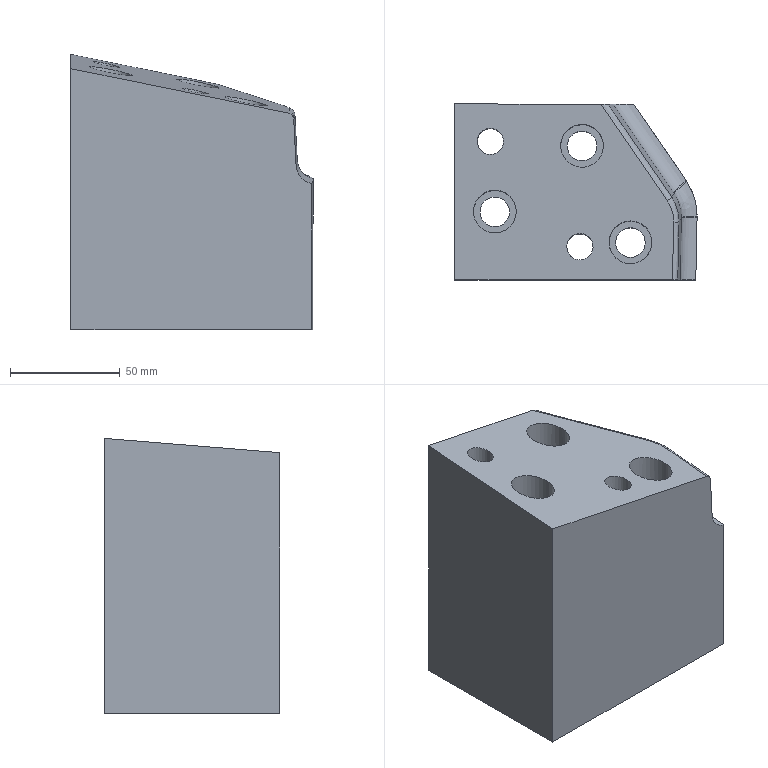Part | NX | features solid 2 | 1 solid | 30 faces | box 110.365 x 80 x 125.43 mm | volume 775159 mm3 | plane 11 | cylinder 11 | spline 8 | commonest cylinder face diameters 13.5 x3 19.5 x3 12 x2 18 x2 40 x1
STEP:
#1=CARTESIAN_POINT('',(-814.169,12.523,30.916));
#2=VERTEX_POINT('',#1);
#3=CARTESIAN_POINT('',(-838.426,48.,38.757));
#4=VERTEX_POINT('',#3);
#5=CARTESIAN_POINT('',(-814.169,12.523,30.916));
#6=CARTESIAN_POINT('',(-815.097,14.059,31.231));
#7=CARTESIAN_POINT('',(-817.162,16.985,31.89));
#8=CARTESIAN_POINT('',(-821.235,22.877,33.202));
#9=CARTESIAN_POINT('',(-826.296,30.263,34.836));
#10=CARTESIAN_POINT('',(-832.36,39.132,36.797));
#11=CARTESIAN_POINT('',(-836.404,45.044,38.104));
#12=CARTESIAN_POINT('',(-838.426,48.,38.757));
#13=B_SPLINE_CURVE_WITH_KNOTS('',3,(#5,#6,#7,#8,#9,#10,#11,#12),.UNSPECIFIED.,.F.,.F.,(4,1,1,1,1,4),(0.0458,0.05136,0.05692,0.06804,0.07916,0.09027),.UNSPECIFIED.);
#14=EDGE_CURVE('',#2,#4,#13,.T.);
#15=ORIENTED_EDGE('',*,*,#14,.T.);
#16=CARTESIAN_POINT('',(-814.56,13.109,31.044));
#17=VERTEX_POINT('',#16);
#18=CARTESIAN_POINT('',(-706.223,-145.27,-3.971));
#19=DIRECTION('',(0.5554,-0.812,-0.1795));
#20=VECTOR('',#19,1000.);
#21=LINE('',#18,#20);
#22=EDGE_CURVE('',#4,#17,#21,.T.);
#23=ORIENTED_EDGE('',*,*,#22,.T.);
#24=CARTESIAN_POINT('',(-838.989,-3.323,34.701));
#25=DIRECTION('',(-0.1996,0.07937,-0.9767));
#26=DIRECTION('',(0.9799,0.02089,-0.1986));
#27=AXIS2_PLACEMENT_3D('',#24,#25,#26);
#28=ELLIPSE('',#27,29.954,29.);
#29=EDGE_CURVE('',#17,#2,#28,.T.);
#30=ORIENTED_EDGE('',*,*,#29,.T.);
#31=EDGE_LOOP('',(#15,#23,#30));
#32=FACE_BOUND('',#31,.T.);
#33=CARTESIAN_POINT('',(-543.724,-28.864,-27.724));
#34=DIRECTION('',(-0.1996,0.07937,-0.9767));
#35=DIRECTION('',(0.9799,0.02089,-0.1986));
#36=AXIS2_PLACEMENT_3D('',#33,#34,#35);
#37=PLANE('',#36);
#38=ADVANCED_FACE('',(#32),#37,.F.);
#39=CARTESIAN_POINT('',(-857.279,-18.669,67.193));
#40=VERTEX_POINT('',#39);
#41=CARTESIAN_POINT('',(-859.902,-22.86,67.388));
#42=CARTESIAN_POINT('',(-856.633,-18.852,67.046));
#43=CARTESIAN_POINT('',(-857.243,-13.746,67.585));
#44=CARTESIAN_POINT('',(-861.169,-10.636,68.641));
#45=CARTESIAN_POINT('',(-866.18,-11.127,69.625));
#46=CARTESIAN_POINT('',(-869.446,-15.132,69.967));
#47=CARTESIAN_POINT('',(-868.843,-20.233,69.429));
#48=CARTESIAN_POINT('',(-864.913,-23.352,68.372));
#49=CARTESIAN_POINT('',(-859.902,-22.86,67.388));
#50=CARTESIAN_POINT('',(-856.633,-18.852,67.046));
#51=CARTESIAN_POINT('',(-857.243,-13.746,67.585));
#52=B_SPLINE_CURVE_WITH_KNOTS('',3,(#41,#42,#43,#44,#45,#46,#47,#48,#49,#50,#51),.UNSPECIFIED.,.T.,.F.,(1,1,1,1,1,1,1,1,1,1,1,1,1,1,1),(-0.01424,-0.009492,-0.004746,0.,0.004746,0.009492,0.01424,0.01898,0.02373,0.02848,0.03322,0.03797,0.04271,0.04746,0.05221),.UNSPECIFIED.);
#53=EDGE_CURVE('',#40,#40,#52,.T.);
#54=ORIENTED_EDGE('',*,*,#53,.F.);
#55=EDGE_LOOP('',(#54));
#56=FACE_BOUND('',#55,.T.);
#57=CARTESIAN_POINT('',(-909.709,-6.673,78.884));
#58=VERTEX_POINT('',#57);
#59=CARTESIAN_POINT('',(-903.612,-11.594,77.238));
#60=CARTESIAN_POINT('',(-910.538,-7.306,79.002));
#61=CARTESIAN_POINT('',(-912.489,0.7824,80.058));
#62=CARTESIAN_POINT('',(-908.008,7.886,79.719));
#63=CARTESIAN_POINT('',(-899.97,9.645,78.219));
#64=CARTESIAN_POINT('',(-893.065,5.359,76.46));
#65=CARTESIAN_POINT('',(-891.101,-2.711,75.402));
#66=CARTESIAN_POINT('',(-895.587,-9.835,75.74));
#67=CARTESIAN_POINT('',(-903.612,-11.594,77.238));
#68=CARTESIAN_POINT('',(-910.538,-7.306,79.002));
#69=CARTESIAN_POINT('',(-912.489,0.7824,80.058));
#70=B_SPLINE_CURVE_WITH_KNOTS('',3,(#59,#60,#61,#62,#63,#64,#65,#66,#67,#68,#69),.UNSPECIFIED.,.T.,.F.,(1,1,1,1,1,1,1,1,1,1,1,1,1,1,1),(-0.02314,-0.01542,-0.007712,0.,0.007712,0.01542,0.02314,0.03085,0.03856,0.04627,0.05398,0.06169,0.06941,0.07712,0.08483),.UNSPECIFIED.);
#71=EDGE_CURVE('',#58,#58,#70,.T.);
#72=ORIENTED_EDGE('',*,*,#71,.T.);
#73=EDGE_LOOP('',(#72));
#74=FACE_BOUND('',#73,.T.);
#75=CARTESIAN_POINT('',(-849.687,-16.103,65.849));
#76=VERTEX_POINT('',#75);
#77=CARTESIAN_POINT('',(-846.7,-23.44,64.643));
#78=CARTESIAN_POINT('',(-850.754,-16.253,66.055));
#79=CARTESIAN_POINT('',(-848.406,-8.168,66.232));
#80=CARTESIAN_POINT('',(-841.091,-4.27,65.054));
#81=CARTESIAN_POINT('',(-833.29,-6.567,63.273));
#82=CARTESIAN_POINT('',(-829.252,-13.743,61.864));
#83=CARTESIAN_POINT('',(-831.581,-21.819,61.684));
#84=CARTESIAN_POINT('',(-838.912,-25.731,62.864));
#85=CARTESIAN_POINT('',(-846.7,-23.44,64.643));
#86=CARTESIAN_POINT('',(-850.754,-16.253,66.055));
#87=CARTESIAN_POINT('',(-848.406,-8.168,66.232));
#88=B_SPLINE_CURVE_WITH_KNOTS('',3,(#77,#78,#79,#80,#81,#82,#83,#84,#85,#86,#87),.UNSPECIFIED.,.T.,.F.,(1,1,1,1,1,1,1,1,1,1,1,1,1,1,1),(-0.02314,-0.01543,-0.007713,0.,0.007713,0.01543,0.02314,0.03085,0.03857,0.04628,0.05399,0.06171,0.06942,0.07713,0.08485),.UNSPECIFIED.);
#89=EDGE_CURVE('',#76,#76,#88,.T.);
#90=ORIENTED_EDGE('',*,*,#89,.T.);
#91=EDGE_LOOP('',(#90));
#92=FACE_BOUND('',#91,.T.);
#93=CARTESIAN_POINT('',(-871.247,25.732,73.656));
#94=VERTEX_POINT('',#93);
#95=CARTESIAN_POINT('',(-866.719,19.289,72.207));
#96=CARTESIAN_POINT('',(-872.237,25.345,73.827));
#97=CARTESIAN_POINT('',(-871.815,33.724,74.421));
#98=CARTESIAN_POINT('',(-865.534,39.227,73.585));
#99=CARTESIAN_POINT('',(-857.389,38.706,71.878));
#100=CARTESIAN_POINT('',(-851.893,32.658,70.263));
#101=CARTESIAN_POINT('',(-852.296,24.292,69.666));
#102=CARTESIAN_POINT('',(-858.589,18.772,70.503));
#103=CARTESIAN_POINT('',(-866.719,19.289,72.207));
#104=CARTESIAN_POINT('',(-872.237,25.345,73.827));
#105=CARTESIAN_POINT('',(-871.815,33.724,74.421));
#106=B_SPLINE_CURVE_WITH_KNOTS('',3,(#95,#96,#97,#98,#99,#100,#101,#102,#103,#104,#105),.UNSPECIFIED.,.T.,.F.,(1,1,1,1,1,1,1,1,1,1,1,1,1,1,1),(-0.02314,-0.01543,-0.007713,0.,0.007713,0.01543,0.02314,0.03085,0.03856,0.04628,0.05399,0.0617,0.06942,0.07713,0.08484),.UNSPECIFIED.);
#107=EDGE_CURVE('',#94,#94,#106,.T.);
#108=ORIENTED_EDGE('',*,*,#107,.T.);
#109=EDGE_LOOP('',(#108));
#110=FACE_BOUND('',#109,.T.);
#111=CARTESIAN_POINT('',(-908.757,34.366,82.024));
#112=VERTEX_POINT('',#111);
#113=CARTESIAN_POINT('',(-904.976,37.499,81.506));
#114=CARTESIAN_POINT('',(-909.304,34.754,82.168));
#115=CARTESIAN_POINT('',(-910.352,29.683,81.97));
#116=CARTESIAN_POINT('',(-907.547,25.48,81.055));
#117=CARTESIAN_POINT('',(-902.655,24.423,79.969));
#118=CARTESIAN_POINT('',(-898.335,27.166,79.309));
#119=CARTESIAN_POINT('',(-897.28,32.228,79.505));
#120=CARTESIAN_POINT('',(-900.089,36.443,80.421));
#121=CARTESIAN_POINT('',(-904.976,37.499,81.506));
#122=CARTESIAN_POINT('',(-909.304,34.754,82.168));
#123=CARTESIAN_POINT('',(-910.352,29.683,81.97));
#124=B_SPLINE_CURVE_WITH_KNOTS('',3,(#113,#114,#115,#116,#117,#118,#119,#120,#121,#122,#123),.UNSPECIFIED.,.T.,.F.,(1,1,1,1,1,1,1,1,1,1,1,1,1,1,1),(-0.01424,-0.009493,-0.004747,0.,0.004747,0.009493,0.01424,0.01899,0.02373,0.02848,0.03323,0.03797,0.04272,0.04747,0.05221),.UNSPECIFIED.);
#125=EDGE_CURVE('',#112,#112,#124,.T.);
#126=ORIENTED_EDGE('',*,*,#125,.F.);
#127=EDGE_LOOP('',(#126));
#128=FACE_BOUND('',#127,.T.);
#129=CARTESIAN_POINT('',(-820.85,-32.,58.663));
#130=VERTEX_POINT('',#129);
#131=CARTESIAN_POINT('',(-920.,-32.,78.929));
#132=VERTEX_POINT('',#131);
#133=CARTESIAN_POINT('',(-820.85,-32.,58.663));
#134=CARTESIAN_POINT('',(-853.9,-32.,65.419));
#135=CARTESIAN_POINT('',(-886.95,-32.,72.174));
#136=CARTESIAN_POINT('',(-920.,-32.,78.929));
#137=B_SPLINE_CURVE_WITH_KNOTS('',3,(#133,#134,#135,#136),.UNSPECIFIED.,.F.,.F.,(4,4),(0.,0.1012),.UNSPECIFIED.);
#138=EDGE_CURVE('',#130,#132,#137,.T.);
#139=ORIENTED_EDGE('',*,*,#138,.F.);
#140=CARTESIAN_POINT('',(-820.322,-5.789,60.686));
#141=VERTEX_POINT('',#140);
#142=CARTESIAN_POINT('',(-820.85,-32.,58.663));
#143=CARTESIAN_POINT('',(-820.674,-23.263,59.337));
#144=CARTESIAN_POINT('',(-820.498,-14.526,60.011));
#145=CARTESIAN_POINT('',(-820.322,-5.789,60.686));
#146=B_SPLINE_CURVE_WITH_KNOTS('',3,(#142,#143,#144,#145),.UNSPECIFIED.,.F.,.F.,(4,4),(0.,0.02629),.UNSPECIFIED.);
#147=EDGE_CURVE('',#130,#141,#146,.T.);
#148=ORIENTED_EDGE('',*,*,#147,.T.);
#149=CARTESIAN_POINT('',(-823.204,3.891,62.061));
#150=VERTEX_POINT('',#149);
#151=CARTESIAN_POINT('',(-820.322,-5.789,60.686));
#152=CARTESIAN_POINT('',(-820.252,-2.318,60.953));
#153=CARTESIAN_POINT('',(-821.27,1.064,61.436));
#154=CARTESIAN_POINT('',(-823.204,3.891,62.061));
#155=B_SPLINE_CURVE_WITH_KNOTS('',3,(#151,#152,#153,#154),.UNSPECIFIED.,.F.,.F.,(4,4),(0.,0.01034),.UNSPECIFIED.);
#156=EDGE_CURVE('',#141,#150,#155,.T.);
#157=ORIENTED_EDGE('',*,*,#156,.T.);
#158=CARTESIAN_POINT('',(-853.376,48.,71.813));
#159=VERTEX_POINT('',#158);
#160=CARTESIAN_POINT('',(-823.204,3.891,62.061));
#161=CARTESIAN_POINT('',(-833.261,18.594,65.312));
#162=CARTESIAN_POINT('',(-843.319,33.297,68.562));
#163=CARTESIAN_POINT('',(-853.376,48.,71.813));
#164=B_SPLINE_CURVE_WITH_KNOTS('',3,(#160,#161,#162,#163),.UNSPECIFIED.,.F.,.F.,(4,4),(0.,0.05432),.UNSPECIFIED.);
#165=EDGE_CURVE('',#150,#159,#164,.T.);
#166=ORIENTED_EDGE('',*,*,#165,.T.);
#167=CARTESIAN_POINT('',(-920.,48.,85.43));
#168=VERTEX_POINT('',#167);
#169=CARTESIAN_POINT('',(-853.376,48.,71.813));
#170=CARTESIAN_POINT('',(-875.584,48.,76.352));
#171=CARTESIAN_POINT('',(-897.792,48.,80.891));
#172=CARTESIAN_POINT('',(-920.,48.,85.43));
#173=B_SPLINE_CURVE_WITH_KNOTS('',3,(#169,#170,#171,#172),.UNSPECIFIED.,.F.,.F.,(4,4),(0.1961,0.2641),.UNSPECIFIED.);
#174=EDGE_CURVE('',#159,#168,#173,.T.);
#175=ORIENTED_EDGE('',*,*,#174,.T.);
#176=CARTESIAN_POINT('',(-920.,-32.,78.929));
#177=CARTESIAN_POINT('',(-920.,-5.333,81.096));
#178=CARTESIAN_POINT('',(-920.,21.333,83.263));
#179=CARTESIAN_POINT('',(-920.,48.,85.43));
#180=B_SPLINE_CURVE_WITH_KNOTS('',3,(#176,#177,#178,#179),.UNSPECIFIED.,.F.,.F.,(4,4),(0.,0.08026),.UNSPECIFIED.);
#181=EDGE_CURVE('',#132,#168,#180,.T.);
#182=ORIENTED_EDGE('',*,*,#181,.F.);
#183=EDGE_LOOP('',(#139,#148,#157,#166,#175,#182));
#184=FACE_BOUND('',#183,.T.);
#185=CARTESIAN_POINT('',(-920.974,48.472,85.668));
#186=CARTESIAN_POINT('',(-920.587,-34.619,78.836));
#187=CARTESIAN_POINT('',(-919.909,48.495,85.452));
#188=CARTESIAN_POINT('',(-919.523,-34.596,78.62));
#189=CARTESIAN_POINT('',(-900.858,48.901,81.591));
#190=CARTESIAN_POINT('',(-900.471,-34.19,74.759));
#191=CARTESIAN_POINT('',(-869.11,49.577,75.157));
#192=CARTESIAN_POINT('',(-868.723,-33.513,68.325));
#193=CARTESIAN_POINT('',(-819.947,50.626,65.194));
#194=CARTESIAN_POINT('',(-819.56,-32.465,58.362));
#195=B_SPLINE_SURFACE_WITH_KNOTS('',1,1,((#185,#186),(#187,#188),(#189,#190),(#191,#192),(#193,#194)),.PLANE_SURF.,.F.,.F.,.F.,(2,1,1,1,2),(2,2),(-0.2849,-0.2791,-0.1744,0.,0.2701),(0.3913,0.7679),.PIECEWISE_BEZIER_KNOTS.);
#196=ADVANCED_FACE('',(#56,#74,#92,#110,#128,#184),#195,.F.);
#197=CARTESIAN_POINT('',(-838.426,48.,-40.));
#198=VERTEX_POINT('',#197);
#199=CARTESIAN_POINT('',(-838.426,48.,-20.));
#200=DIRECTION('',(0.,0.,1.));
#201=VECTOR('',#200,1000.);
#202=LINE('',#199,#201);
#203=EDGE_CURVE('',#4,#198,#202,.F.);
#204=ORIENTED_EDGE('',*,*,#203,.F.);
#205=ORIENTED_EDGE('',*,*,#14,.F.);
#206=CARTESIAN_POINT('',(-809.639,-2.963,28.732));
#207=VERTEX_POINT('',#206);
#208=CARTESIAN_POINT('',(-809.639,-2.963,28.732));
#209=CARTESIAN_POINT('',(-809.665,-0.1967,28.962));
#210=CARTESIAN_POINT('',(-810.39,5.202,29.549));
#211=CARTESIAN_POINT('',(-812.779,10.219,30.445));
#212=CARTESIAN_POINT('',(-814.169,12.523,30.916));
#213=B_SPLINE_CURVE_WITH_KNOTS('',3,(#208,#209,#210,#211,#212),.UNSPECIFIED.,.F.,.F.,(4,1,4),(0.02913,0.03746,0.0458),.UNSPECIFIED.);
#214=EDGE_CURVE('',#207,#2,#213,.T.);
#215=ORIENTED_EDGE('',*,*,#214,.F.);
#216=CARTESIAN_POINT('',(-810.22,-32.,26.491));
#217=VERTEX_POINT('',#216);
#218=CARTESIAN_POINT('',(-810.22,-32.,26.491));
#219=CARTESIAN_POINT('',(-810.123,-27.16,26.864));
#220=CARTESIAN_POINT('',(-809.961,-19.9,27.421));
#221=CARTESIAN_POINT('',(-809.807,-10.223,28.176));
#222=CARTESIAN_POINT('',(-809.615,-5.38,28.53));
#223=CARTESIAN_POINT('',(-809.639,-2.963,28.732));
#224=B_SPLINE_CURVE_WITH_KNOTS('',3,(#218,#219,#220,#221,#222,#223),.UNSPECIFIED.,.F.,.F.,(4,1,1,4),(0.,0.01456,0.02185,0.02913),.UNSPECIFIED.);
#225=EDGE_CURVE('',#217,#207,#224,.T.);
#226=ORIENTED_EDGE('',*,*,#225,.F.);
#227=CARTESIAN_POINT('',(-810.22,-32.,-40.));
#228=VERTEX_POINT('',#227);
#229=CARTESIAN_POINT('',(-810.22,-32.,-20.));
#230=DIRECTION('',(0.,0.,1.));
#231=VECTOR('',#230,1000.);
#232=LINE('',#229,#231);
#233=EDGE_CURVE('',#217,#228,#232,.F.);
#234=ORIENTED_EDGE('',*,*,#233,.T.);
#235=CARTESIAN_POINT('',(-810.22,-32.,-40.));
#236=CARTESIAN_POINT('',(-810.146,-28.288,-40.));
#237=CARTESIAN_POINT('',(-810.036,-22.72,-40.));
#238=CARTESIAN_POINT('',(-809.879,-15.297,-40.));
#239=CARTESIAN_POINT('',(-809.787,-9.727,-40.));
#240=CARTESIAN_POINT('',(-809.579,-4.166,-40.));
#241=CARTESIAN_POINT('',(-809.762,1.427,-40.));
#242=CARTESIAN_POINT('',(-811.176,6.752,-40.));
#243=CARTESIAN_POINT('',(-813.579,11.806,-40.));
#244=CARTESIAN_POINT('',(-816.679,16.319,-40.));
#245=CARTESIAN_POINT('',(-819.822,20.825,-40.));
#246=CARTESIAN_POINT('',(-822.929,25.349,-40.));
#247=CARTESIAN_POINT('',(-827.065,31.388,-40.));
#248=CARTESIAN_POINT('',(-832.228,38.939,-40.));
#249=CARTESIAN_POINT('',(-836.36,44.98,-40.));
#250=CARTESIAN_POINT('',(-838.426,48.,-40.));
#251=B_SPLINE_CURVE_WITH_KNOTS('',3,(#235,#236,#237,#238,#239,#240,#241,#242,#243,#244,#245,#246,#247,#248,#249,#250),.UNSPECIFIED.,.F.,.F.,(4,1,1,1,1,1,1,1,1,1,1,1,1,4),(0.,0.01114,0.01671,0.02228,0.02784,0.03341,0.03898,0.04455,0.05012,0.05569,0.06126,0.06683,0.07797,0.0891),.UNSPECIFIED.);
#252=EDGE_CURVE('',#228,#198,#251,.T.);
#253=ORIENTED_EDGE('',*,*,#252,.T.);
#254=EDGE_LOOP('',(#204,#205,#215,#226,#234,#253));
#255=FACE_BOUND('',#254,.T.);
#256=CARTESIAN_POINT('',(-838.426,48.,-40.));
#257=CARTESIAN_POINT('',(-838.426,48.,39.23));
#258=CARTESIAN_POINT('',(-834.685,42.53,-40.));
#259=CARTESIAN_POINT('',(-834.685,42.53,39.23));
#260=CARTESIAN_POINT('',(-827.52,32.055,-40.));
#261=CARTESIAN_POINT('',(-827.52,32.055,39.23));
#262=CARTESIAN_POINT('',(-819.564,20.425,-40.));
#263=CARTESIAN_POINT('',(-819.564,20.425,39.23));
#264=CARTESIAN_POINT('',(-813.609,11.918,-40.));
#265=CARTESIAN_POINT('',(-813.609,11.918,39.23));
#266=CARTESIAN_POINT('',(-811.044,6.684,-40.));
#267=CARTESIAN_POINT('',(-811.044,6.684,39.23));
#268=CARTESIAN_POINT('',(-809.788,0.9757,-40.));
#269=CARTESIAN_POINT('',(-809.788,0.9757,39.23));
#270=CARTESIAN_POINT('',(-809.603,-2.547,-40.));
#271=CARTESIAN_POINT('',(-809.603,-2.547,39.23));
#272=CARTESIAN_POINT('',(-809.753,-8.818,-40.));
#273=CARTESIAN_POINT('',(-809.753,-8.818,39.23));
#274=CARTESIAN_POINT('',(-809.945,-18.35,-40.));
#275=CARTESIAN_POINT('',(-809.945,-18.35,39.23));
#276=CARTESIAN_POINT('',(-810.125,-27.28,-40.));
#277=CARTESIAN_POINT('',(-810.125,-27.28,39.23));
#278=CARTESIAN_POINT('',(-810.22,-32.,-40.));
#279=CARTESIAN_POINT('',(-810.22,-32.,39.23));
#280=B_SPLINE_SURFACE_WITH_KNOTS('',3,1,((#256,#257),(#258,#259),(#260,#261),(#262,#263),(#264,#265),(#266,#267),(#268,#269),(#270,#271),(#272,#273),(#274,#275),(#276,#277),(#278,#279)),.SURF_OF_LINEAR_EXTRUSION.,.F.,.F.,.F.,(4,1,1,1,1,1,1,1,1,4),(2,2),(0.4314,0.463,0.492,0.4987,0.5127,0.5196,0.5266,0.5295,0.5496,0.5722),(0.4274,0.7151),.UNSPECIFIED.);
#281=ADVANCED_FACE('',(#255),#280,.F.);
#282=ORIENTED_EDGE('',*,*,#174,.F.);
#283=CARTESIAN_POINT('',(-850.192,48.,68.733));
#284=VERTEX_POINT('',#283);
#285=CARTESIAN_POINT('',(-853.376,48.,71.813));
#286=CARTESIAN_POINT('',(-852.599,48.,71.654));
#287=CARTESIAN_POINT('',(-851.15,48.,70.951));
#288=CARTESIAN_POINT('',(-850.277,48.,69.525));
#289=CARTESIAN_POINT('',(-850.192,48.,68.733));
#290=B_SPLINE_CURVE_WITH_KNOTS('',3,(#285,#286,#287,#288,#289),.UNSPECIFIED.,.F.,.F.,(4,1,4),(0.,0.002346,0.004693),.UNSPECIFIED.);
#291=EDGE_CURVE('',#159,#284,#290,.T.);
#292=ORIENTED_EDGE('',*,*,#291,.T.);
#293=CARTESIAN_POINT('',(-847.978,48.,47.999));
#294=VERTEX_POINT('',#293);
#295=CARTESIAN_POINT('',(-838.657,48.,-39.294));
#296=DIRECTION('',(-0.1062,0.,0.9943));
#297=VECTOR('',#296,1000.);
#298=LINE('',#295,#297);
#299=EDGE_CURVE('',#284,#294,#298,.F.);
#300=ORIENTED_EDGE('',*,*,#299,.T.);
#301=CARTESIAN_POINT('',(-837.118,48.,47.705));
#302=DIRECTION('',(0.,1.,0.));
#303=DIRECTION('',(-0.9515,0.,0.3075));
#304=AXIS2_PLACEMENT_3D('',#301,#302,#303);
#305=ELLIPSE('',#304,11.084,9.);
#306=EDGE_CURVE('',#294,#4,#305,.F.);
#307=ORIENTED_EDGE('',*,*,#306,.T.);
#308=ORIENTED_EDGE('',*,*,#203,.T.);
#309=CARTESIAN_POINT('',(-920.,48.,-40.));
#310=VERTEX_POINT('',#309);
#311=CARTESIAN_POINT('',(-813.69,48.,-40.));
#312=DIRECTION('',(1.,0.,0.));
#313=VECTOR('',#312,1000.);
#314=LINE('',#311,#313);
#315=EDGE_CURVE('',#198,#310,#314,.F.);
#316=ORIENTED_EDGE('',*,*,#315,.T.);
#317=CARTESIAN_POINT('',(-920.,48.,100.));
#318=DIRECTION('',(0.,0.,1.));
#319=VECTOR('',#318,1000.);
#320=LINE('',#317,#319);
#321=EDGE_CURVE('',#168,#310,#320,.F.);
#322=ORIENTED_EDGE('',*,*,#321,.F.);
#323=EDGE_LOOP('',(#282,#292,#300,#307,#308,#316,#322));
#324=FACE_BOUND('',#323,.T.);
#325=CARTESIAN_POINT('',(-915.5,48.,-47.5));
#326=DIRECTION('',(0.,1.,0.));
#327=DIRECTION('',(-1.,0.,0.));
#328=AXIS2_PLACEMENT_3D('',#325,#326,#327);
#329=PLANE('',#328);
#330=ADVANCED_FACE('',(#324),#329,.T.);
#331=CARTESIAN_POINT('',(-817.4,-32.,34.867));
#332=VERTEX_POINT('',#331);
#333=CARTESIAN_POINT('',(-818.457,-32.,55.871));
#334=VERTEX_POINT('',#333);
#335=CARTESIAN_POINT('',(-813.512,-32.,-42.366));
#336=DIRECTION('',(0.05028,0.,-0.9987));
#337=VECTOR('',#336,1000.);
#338=LINE('',#335,#337);
#339=EDGE_CURVE('',#332,#334,#338,.F.);
#340=ORIENTED_EDGE('',*,*,#339,.T.);
#341=CARTESIAN_POINT('',(-818.457,-32.,55.871));
#342=CARTESIAN_POINT('',(-818.524,-32.,57.201));
#343=CARTESIAN_POINT('',(-819.546,-32.,58.397));
#344=CARTESIAN_POINT('',(-820.85,-32.,58.663));
#345=B_SPLINE_CURVE_WITH_KNOTS('',3,(#341,#342,#343,#344),.UNSPECIFIED.,.F.,.F.,(4,4),(0.,0.003938),.UNSPECIFIED.);
#346=EDGE_CURVE('',#334,#130,#345,.T.);
#347=ORIENTED_EDGE('',*,*,#346,.T.);
#348=ORIENTED_EDGE('',*,*,#138,.T.);
#349=CARTESIAN_POINT('',(-920.,-32.,-40.));
#350=VERTEX_POINT('',#349);
#351=CARTESIAN_POINT('',(-920.,-32.,100.));
#352=DIRECTION('',(0.,0.,-1.));
#353=VECTOR('',#352,1000.);
#354=LINE('',#351,#353);
#355=EDGE_CURVE('',#132,#350,#354,.T.);
#356=ORIENTED_EDGE('',*,*,#355,.T.);
#357=CARTESIAN_POINT('',(-813.69,-32.,-40.));
#358=DIRECTION('',(-1.,0.,0.));
#359=VECTOR('',#358,1000.);
#360=LINE('',#357,#359);
#361=EDGE_CURVE('',#228,#350,#360,.T.);
#362=ORIENTED_EDGE('',*,*,#361,.F.);
#363=ORIENTED_EDGE('',*,*,#233,.F.);
#364=CARTESIAN_POINT('',(-808.409,-32.,35.336));
#365=DIRECTION('',(0.,-1.,0.));
#366=DIRECTION('',(0.2528,0.,0.9675));
#367=AXIS2_PLACEMENT_3D('',#364,#365,#366);
#368=ELLIPSE('',#367,9.029,9.);
#369=EDGE_CURVE('',#217,#332,#368,.F.);
#370=ORIENTED_EDGE('',*,*,#369,.T.);
#371=EDGE_LOOP('',(#340,#347,#348,#356,#362,#363,#370));
#372=FACE_BOUND('',#371,.T.);
#373=CARTESIAN_POINT('',(-915.5,-32.,-47.5));
#374=DIRECTION('',(0.,-1.,0.));
#375=DIRECTION('',(1.,0.,0.));
#376=AXIS2_PLACEMENT_3D('',#373,#374,#375);
#377=PLANE('',#376);
#378=ADVANCED_FACE('',(#372),#377,.T.);
#379=ORIENTED_EDGE('',*,*,#252,.F.);
#380=ORIENTED_EDGE('',*,*,#361,.T.);
#381=CARTESIAN_POINT('',(-920.,-31.695,-40.));
#382=DIRECTION('',(0.,1.,0.));
#383=VECTOR('',#382,1000.);
#384=LINE('',#381,#383);
#385=EDGE_CURVE('',#350,#310,#384,.T.);
#386=ORIENTED_EDGE('',*,*,#385,.T.);
#387=ORIENTED_EDGE('',*,*,#315,.F.);
#388=EDGE_LOOP('',(#379,#380,#386,#387));
#389=FACE_BOUND('',#388,.T.);
#390=CARTESIAN_POINT('',(-869.041,-16.993,-40.));
#391=VERTEX_POINT('',#390);
#392=CARTESIAN_POINT('',(-863.041,-16.993,-40.));
#393=DIRECTION('',(0.,0.,-1.));
#394=DIRECTION('',(-1.,0.,0.));
#395=AXIS2_PLACEMENT_3D('',#392,#393,#394);
#396=CIRCLE('',#395,6.);
#397=EDGE_CURVE('',#391,#391,#396,.F.);
#398=ORIENTED_EDGE('',*,*,#397,.T.);
#399=EDGE_LOOP('',(#398));
#400=FACE_BOUND('',#399,.T.);
#401=CARTESIAN_POINT('',(-908.547,-0.9737,-40.));
#402=VERTEX_POINT('',#401);
#403=CARTESIAN_POINT('',(-901.797,-0.9737,-40.));
#404=DIRECTION('',(0.,0.,-1.));
#405=DIRECTION('',(-1.,0.,0.));
#406=AXIS2_PLACEMENT_3D('',#403,#404,#405);
#407=CIRCLE('',#406,6.75);
#408=EDGE_CURVE('',#402,#402,#407,.T.);
#409=ORIENTED_EDGE('',*,*,#408,.F.);
#410=EDGE_LOOP('',(#409));
#411=FACE_BOUND('',#410,.T.);
#412=CARTESIAN_POINT('',(-846.75,-15.,-40.));
#413=VERTEX_POINT('',#412);
#414=CARTESIAN_POINT('',(-840.,-15.,-40.));
#415=DIRECTION('',(0.,0.,-1.));
#416=DIRECTION('',(-1.,0.,0.));
#417=AXIS2_PLACEMENT_3D('',#414,#415,#416);
#418=CIRCLE('',#417,6.75);
#419=EDGE_CURVE('',#413,#413,#418,.T.);
#420=ORIENTED_EDGE('',*,*,#419,.F.);
#421=EDGE_LOOP('',(#420));
#422=FACE_BOUND('',#421,.T.);
#423=CARTESIAN_POINT('',(-868.811,29.,-40.));
#424=VERTEX_POINT('',#423);
#425=CARTESIAN_POINT('',(-862.061,29.,-40.));
#426=DIRECTION('',(0.,0.,-1.));
#427=DIRECTION('',(-1.,0.,0.));
#428=AXIS2_PLACEMENT_3D('',#425,#426,#427);
#429=CIRCLE('',#428,6.75);
#430=EDGE_CURVE('',#424,#424,#429,.T.);
#431=ORIENTED_EDGE('',*,*,#430,.F.);
#432=EDGE_LOOP('',(#431));
#433=FACE_BOUND('',#432,.T.);
#434=CARTESIAN_POINT('',(-909.818,30.961,-40.));
#435=VERTEX_POINT('',#434);
#436=CARTESIAN_POINT('',(-903.818,30.961,-40.));
#437=DIRECTION('',(0.,0.,-1.));
#438=DIRECTION('',(-1.,0.,0.));
#439=AXIS2_PLACEMENT_3D('',#436,#437,#438);
#440=CIRCLE('',#439,6.);
#441=EDGE_CURVE('',#435,#435,#440,.F.);
#442=ORIENTED_EDGE('',*,*,#441,.T.);
#443=EDGE_LOOP('',(#442));
#444=FACE_BOUND('',#443,.T.);
#445=CARTESIAN_POINT('',(-813.69,4.103,-40.));
#446=DIRECTION('',(0.,0.,-1.));
#447=DIRECTION('',(-1.,0.,0.));
#448=AXIS2_PLACEMENT_3D('',#445,#446,#447);
#449=PLANE('',#448);
#450=ADVANCED_FACE('',(#389,#400,#411,#422,#433,#444),#449,.T.);
#451=ORIENTED_EDGE('',*,*,#385,.F.);
#452=ORIENTED_EDGE('',*,*,#355,.F.);
#453=ORIENTED_EDGE('',*,*,#181,.T.);
#454=ORIENTED_EDGE('',*,*,#321,.T.);
#455=EDGE_LOOP('',(#451,#452,#453,#454));
#456=FACE_BOUND('',#455,.T.);
#457=CARTESIAN_POINT('',(-920.,-31.695,100.));
#458=DIRECTION('',(1.,0.,0.));
#459=DIRECTION('',(0.,0.,1.));
#460=AXIS2_PLACEMENT_3D('',#457,#458,#459);
#461=PLANE('',#460);
#462=ADVANCED_FACE('',(#456),#461,.F.);
#463=CARTESIAN_POINT('',(-871.811,29.,-25.));
#464=VERTEX_POINT('',#463);
#465=CARTESIAN_POINT('',(-862.061,29.,-25.));
#466=DIRECTION('',(0.,0.,-1.));
#467=DIRECTION('',(-1.,0.,0.));
#468=AXIS2_PLACEMENT_3D('',#465,#466,#467);
#469=CIRCLE('',#468,9.75);
#470=EDGE_CURVE('',#464,#464,#469,.F.);
#471=ORIENTED_EDGE('',*,*,#470,.F.);
#472=EDGE_LOOP('',(#471));
#473=FACE_BOUND('',#472,.T.);
#474=ORIENTED_EDGE('',*,*,#107,.F.);
#475=EDGE_LOOP('',(#474));
#476=FACE_BOUND('',#475,.T.);
#477=CARTESIAN_POINT('',(-862.061,29.,-26.006));
#478=DIRECTION('',(0.,0.,1.));
#479=DIRECTION('',(1.,0.,0.));
#480=AXIS2_PLACEMENT_3D('',#477,#478,#479);
#481=CYLINDRICAL_SURFACE('',#480,9.75);
#482=ADVANCED_FACE('',(#473,#476),#481,.F.);
#483=ORIENTED_EDGE('',*,*,#430,.T.);
#484=EDGE_LOOP('',(#483));
#485=FACE_BOUND('',#484,.T.);
#486=CARTESIAN_POINT('',(-868.811,29.,-25.));
#487=VERTEX_POINT('',#486);
#488=CARTESIAN_POINT('',(-862.061,29.,-25.));
#489=DIRECTION('',(0.,0.,-1.));
#490=DIRECTION('',(-1.,0.,0.));
#491=AXIS2_PLACEMENT_3D('',#488,#489,#490);
#492=CIRCLE('',#491,6.75);
#493=EDGE_CURVE('',#487,#487,#492,.F.);
#494=ORIENTED_EDGE('',*,*,#493,.T.);
#495=EDGE_LOOP('',(#494));
#496=FACE_BOUND('',#495,.T.);
#497=CARTESIAN_POINT('',(-862.061,29.,-56.006));
#498=DIRECTION('',(0.,0.,1.));
#499=DIRECTION('',(1.,0.,0.));
#500=AXIS2_PLACEMENT_3D('',#497,#498,#499);
#501=CYLINDRICAL_SURFACE('',#500,6.75);
#502=ADVANCED_FACE('',(#485,#496),#501,.F.);
#503=ORIENTED_EDGE('',*,*,#493,.F.);
#504=EDGE_LOOP('',(#503));
#505=FACE_BOUND('',#504,.T.);
#506=ORIENTED_EDGE('',*,*,#470,.T.);
#507=EDGE_LOOP('',(#506));
#508=FACE_BOUND('',#507,.T.);
#509=CARTESIAN_POINT('',(-863.613,34.418,-25.));
#510=DIRECTION('',(0.,0.,-1.));
#511=DIRECTION('',(-1.,0.,0.));
#512=AXIS2_PLACEMENT_3D('',#509,#510,#511);
#513=PLANE('',#512);
#514=ADVANCED_FACE('',(#505,#508),#513,.F.);
#515=CARTESIAN_POINT('',(-830.25,-15.,-25.));
#516=VERTEX_POINT('',#515);
#517=CARTESIAN_POINT('',(-840.,-15.,-25.));
#518=DIRECTION('',(0.,0.,1.));
#519=DIRECTION('',(1.,0.,0.));
#520=AXIS2_PLACEMENT_3D('',#517,#518,#519);
#521=CIRCLE('',#520,9.75);
#522=EDGE_CURVE('',#516,#516,#521,.T.);
#523=ORIENTED_EDGE('',*,*,#522,.F.);
#524=EDGE_LOOP('',(#523));
#525=FACE_BOUND('',#524,.T.);
#526=ORIENTED_EDGE('',*,*,#89,.F.);
#527=EDGE_LOOP('',(#526));
#528=FACE_BOUND('',#527,.T.);
#529=CARTESIAN_POINT('',(-840.,-15.,-25.));
#530=DIRECTION('',(0.,0.,1.));
#531=DIRECTION('',(1.,0.,0.));
#532=AXIS2_PLACEMENT_3D('',#529,#530,#531);
#533=CYLINDRICAL_SURFACE('',#532,9.75);
#534=ADVANCED_FACE('',(#525,#528),#533,.F.);
#535=ORIENTED_EDGE('',*,*,#419,.T.);
#536=EDGE_LOOP('',(#535));
#537=FACE_BOUND('',#536,.T.);
#538=CARTESIAN_POINT('',(-846.75,-15.,-25.));
#539=VERTEX_POINT('',#538);
#540=CARTESIAN_POINT('',(-840.,-15.,-25.));
#541=DIRECTION('',(0.,0.,-1.));
#542=DIRECTION('',(-1.,0.,0.));
#543=AXIS2_PLACEMENT_3D('',#540,#541,#542);
#544=CIRCLE('',#543,6.75);
#545=EDGE_CURVE('',#539,#539,#544,.F.);
#546=ORIENTED_EDGE('',*,*,#545,.T.);
#547=EDGE_LOOP('',(#546));
#548=FACE_BOUND('',#547,.T.);
#549=CARTESIAN_POINT('',(-840.,-15.,-55.));
#550=DIRECTION('',(0.,0.,1.));
#551=DIRECTION('',(1.,0.,0.));
#552=AXIS2_PLACEMENT_3D('',#549,#550,#551);
#553=CYLINDRICAL_SURFACE('',#552,6.75);
#554=ADVANCED_FACE('',(#537,#548),#553,.F.);
#555=ORIENTED_EDGE('',*,*,#545,.F.);
#556=EDGE_LOOP('',(#555));
#557=FACE_BOUND('',#556,.T.);
#558=ORIENTED_EDGE('',*,*,#522,.T.);
#559=EDGE_LOOP('',(#558));
#560=FACE_BOUND('',#559,.T.);
#561=CARTESIAN_POINT('',(-839.305,-14.502,-25.));
#562=DIRECTION('',(0.,0.,-1.));
#563=DIRECTION('',(-1.,0.,0.));
#564=AXIS2_PLACEMENT_3D('',#561,#562,#563);
#565=PLANE('',#564);
#566=ADVANCED_FACE('',(#557,#560),#565,.F.);
#567=CARTESIAN_POINT('',(-911.547,-0.9737,-25.));
#568=VERTEX_POINT('',#567);
#569=CARTESIAN_POINT('',(-901.797,-0.9737,-25.));
#570=DIRECTION('',(0.,0.,-1.));
#571=DIRECTION('',(-1.,0.,0.));
#572=AXIS2_PLACEMENT_3D('',#569,#570,#571);
#573=CIRCLE('',#572,9.75);
#574=EDGE_CURVE('',#568,#568,#573,.F.);
#575=ORIENTED_EDGE('',*,*,#574,.F.);
#576=EDGE_LOOP('',(#575));
#577=FACE_BOUND('',#576,.T.);
#578=ORIENTED_EDGE('',*,*,#71,.F.);
#579=EDGE_LOOP('',(#578));
#580=FACE_BOUND('',#579,.T.);
#581=CARTESIAN_POINT('',(-901.797,-0.9737,-23.645));
#582=DIRECTION('',(0.,0.,1.));
#583=DIRECTION('',(1.,0.,0.));
#584=AXIS2_PLACEMENT_3D('',#581,#582,#583);
#585=CYLINDRICAL_SURFACE('',#584,9.75);
#586=ADVANCED_FACE('',(#577,#580),#585,.F.);
#587=ORIENTED_EDGE('',*,*,#408,.T.);
#588=EDGE_LOOP('',(#587));
#589=FACE_BOUND('',#588,.T.);
#590=CARTESIAN_POINT('',(-908.547,-0.9737,-25.));
#591=VERTEX_POINT('',#590);
#592=CARTESIAN_POINT('',(-901.797,-0.9737,-25.));
#593=DIRECTION('',(0.,0.,-1.));
#594=DIRECTION('',(-1.,0.,0.));
#595=AXIS2_PLACEMENT_3D('',#592,#593,#594);
#596=CIRCLE('',#595,6.75);
#597=EDGE_CURVE('',#591,#591,#596,.F.);
#598=ORIENTED_EDGE('',*,*,#597,.T.);
#599=EDGE_LOOP('',(#598));
#600=FACE_BOUND('',#599,.T.);
#601=CARTESIAN_POINT('',(-901.797,-0.9737,-53.645));
#602=DIRECTION('',(0.,0.,1.));
#603=DIRECTION('',(1.,0.,0.));
#604=AXIS2_PLACEMENT_3D('',#601,#602,#603);
#605=CYLINDRICAL_SURFACE('',#604,6.75);
#606=ADVANCED_FACE('',(#589,#600),#605,.F.);
#607=ORIENTED_EDGE('',*,*,#597,.F.);
#608=EDGE_LOOP('',(#607));
#609=FACE_BOUND('',#608,.T.);
#610=ORIENTED_EDGE('',*,*,#574,.T.);
#611=EDGE_LOOP('',(#610));
#612=FACE_BOUND('',#611,.T.);
#613=CARTESIAN_POINT('',(-891.236,6.16,-25.));
#614=DIRECTION('',(0.,0.,-1.));
#615=DIRECTION('',(-1.,0.,0.));
#616=AXIS2_PLACEMENT_3D('',#613,#614,#615);
#617=PLANE('',#616);
#618=ADVANCED_FACE('',(#609,#612),#617,.F.);
#619=ORIENTED_EDGE('',*,*,#397,.F.);
#620=EDGE_LOOP('',(#619));
#621=FACE_BOUND('',#620,.T.);
#622=ORIENTED_EDGE('',*,*,#53,.T.);
#623=EDGE_LOOP('',(#622));
#624=FACE_BOUND('',#623,.T.);
#625=CARTESIAN_POINT('',(-863.041,-16.993,459.437));
#626=DIRECTION('',(0.,0.,-1.));
#627=DIRECTION('',(-1.,0.,0.));
#628=AXIS2_PLACEMENT_3D('',#625,#626,#627);
#629=CYLINDRICAL_SURFACE('',#628,6.);
#630=ADVANCED_FACE('',(#621,#624),#629,.F.);
#631=ORIENTED_EDGE('',*,*,#441,.F.);
#632=EDGE_LOOP('',(#631));
#633=FACE_BOUND('',#632,.T.);
#634=ORIENTED_EDGE('',*,*,#125,.T.);
#635=EDGE_LOOP('',(#634));
#636=FACE_BOUND('',#635,.T.);
#637=CARTESIAN_POINT('',(-903.818,30.961,462.774));
#638=DIRECTION('',(0.,0.,-1.));
#639=DIRECTION('',(-1.,0.,0.));
#640=AXIS2_PLACEMENT_3D('',#637,#638,#639);
#641=CYLINDRICAL_SURFACE('',#640,6.);
#642=ADVANCED_FACE('',(#633,#636),#641,.F.);
#643=ORIENTED_EDGE('',*,*,#225,.T.);
#644=CARTESIAN_POINT('',(-809.644,-3.404,28.697));
#645=VERTEX_POINT('',#644);
#646=CARTESIAN_POINT('',(-838.989,-3.323,34.701));
#647=DIRECTION('',(-0.1996,0.07937,-0.9767));
#648=DIRECTION('',(0.9799,0.02089,-0.1986));
#649=AXIS2_PLACEMENT_3D('',#646,#647,#648);
#650=ELLIPSE('',#649,29.954,29.);
#651=EDGE_CURVE('',#207,#645,#650,.T.);
#652=ORIENTED_EDGE('',*,*,#651,.T.);
#653=CARTESIAN_POINT('',(-810.134,-27.703,26.822));
#654=DIRECTION('',(-0.02009,-0.9968,-0.07691));
#655=VECTOR('',#654,1000.);
#656=LINE('',#653,#655);
#657=EDGE_CURVE('',#645,#217,#656,.T.);
#658=ORIENTED_EDGE('',*,*,#657,.T.);
#659=EDGE_LOOP('',(#643,#652,#658));
#660=FACE_BOUND('',#659,.T.);
#661=CARTESIAN_POINT('',(-543.724,-28.864,-27.724));
#662=DIRECTION('',(-0.1996,0.07937,-0.9767));
#663=DIRECTION('',(0.9799,0.02089,-0.1986));
#664=AXIS2_PLACEMENT_3D('',#661,#662,#663);
#665=PLANE('',#664);
#666=ADVANCED_FACE('',(#660),#665,.F.);
#667=CARTESIAN_POINT('',(-817.926,-5.623,57.906));
#668=VERTEX_POINT('',#667);
#669=CARTESIAN_POINT('',(-816.833,-3.902,37.034));
#670=VERTEX_POINT('',#669);
#671=CARTESIAN_POINT('',(-817.052,-4.247,41.211));
#672=DIRECTION('',(0.05208,0.08207,-0.9953));
#673=VECTOR('',#672,1000.);
#674=LINE('',#671,#673);
#675=EDGE_CURVE('',#668,#670,#674,.T.);
#676=ORIENTED_EDGE('',*,*,#675,.F.);
#677=CARTESIAN_POINT('',(-817.926,-5.623,57.906));
#678=CARTESIAN_POINT('',(-818.103,-14.416,57.228));
#679=CARTESIAN_POINT('',(-818.28,-23.208,56.55));
#680=CARTESIAN_POINT('',(-818.457,-32.,55.871));
#681=B_SPLINE_CURVE_WITH_KNOTS('',3,(#677,#678,#679,#680),.UNSPECIFIED.,.F.,.F.,(4,4),(0.,0.02646),.UNSPECIFIED.);
#682=EDGE_CURVE('',#668,#334,#681,.T.);
#683=ORIENTED_EDGE('',*,*,#682,.T.);
#684=ORIENTED_EDGE('',*,*,#339,.F.);
#685=CARTESIAN_POINT('',(-817.737,-48.75,33.574));
#686=DIRECTION('',(0.02009,0.9968,0.07691));
#687=VECTOR('',#686,1000.);
#688=LINE('',#685,#687);
#689=EDGE_CURVE('',#332,#670,#688,.T.);
#690=ORIENTED_EDGE('',*,*,#689,.T.);
#691=EDGE_LOOP('',(#676,#683,#684,#690));
#692=FACE_BOUND('',#691,.T.);
#693=CARTESIAN_POINT('',(-817.941,-49.046,37.471));
#694=DIRECTION('',(-0.9984,0.024,-0.05026));
#695=DIRECTION('',(0.01976,0.9963,0.0832));
#696=AXIS2_PLACEMENT_3D('',#693,#694,#695);
#697=PLANE('',#696);
#698=ADVANCED_FACE('',(#692),#697,.F.);
#699=ORIENTED_EDGE('',*,*,#299,.F.);
#700=CARTESIAN_POINT('',(-821.309,5.775,59.398));
#701=VERTEX_POINT('',#700);
#702=CARTESIAN_POINT('',(-850.192,48.,68.733));
#703=CARTESIAN_POINT('',(-840.565,33.925,65.621));
#704=CARTESIAN_POINT('',(-830.937,19.85,62.509));
#705=CARTESIAN_POINT('',(-821.309,5.775,59.398));
#706=B_SPLINE_CURVE_WITH_KNOTS('',3,(#702,#703,#704,#705),.UNSPECIFIED.,.F.,.F.,(4,4),(0.,0.052),.UNSPECIFIED.);
#707=EDGE_CURVE('',#284,#701,#706,.T.);
#708=ORIENTED_EDGE('',*,*,#707,.T.);
#709=CARTESIAN_POINT('',(-820.244,7.455,39.035));
#710=VERTEX_POINT('',#709);
#711=CARTESIAN_POINT('',(-820.398,7.212,41.981));
#712=DIRECTION('',(-0.05208,-0.08207,0.9953));
#713=VECTOR('',#712,1000.);
#714=LINE('',#711,#713);
#715=EDGE_CURVE('',#710,#701,#714,.T.);
#716=ORIENTED_EDGE('',*,*,#715,.F.);
#717=CARTESIAN_POINT('',(-820.475,7.793,39.11));
#718=DIRECTION('',(-0.5554,0.812,0.1795));
#719=VECTOR('',#718,1000.);
#720=LINE('',#717,#719);
#721=EDGE_CURVE('',#710,#294,#720,.T.);
#722=ORIENTED_EDGE('',*,*,#721,.T.);
#723=EDGE_LOOP('',(#699,#708,#716,#722));
#724=FACE_BOUND('',#723,.T.);
#725=CARTESIAN_POINT('',(-820.398,7.212,41.981));
#726=DIRECTION('',(-0.8312,-0.5489,-0.08875));
#727=DIRECTION('',(-0.5536,0.8318,0.03963));
#728=AXIS2_PLACEMENT_3D('',#725,#726,#727);
#729=PLANE('',#728);
#730=ADVANCED_FACE('',(#724),#729,.F.);
#731=ORIENTED_EDGE('',*,*,#715,.T.);
#732=CARTESIAN_POINT('',(-821.309,5.775,59.398));
#733=CARTESIAN_POINT('',(-819.035,2.437,58.747));
#734=CARTESIAN_POINT('',(-817.844,-1.544,58.225));
#735=CARTESIAN_POINT('',(-817.926,-5.623,57.906));
#736=B_SPLINE_CURVE_WITH_KNOTS('',3,(#732,#733,#734,#735),.UNSPECIFIED.,.F.,.F.,(4,4),(0.,0.01211),.UNSPECIFIED.);
#737=EDGE_CURVE('',#701,#668,#736,.T.);
#738=ORIENTED_EDGE('',*,*,#737,.T.);
#739=ORIENTED_EDGE('',*,*,#675,.T.);
#740=CARTESIAN_POINT('',(-816.83,-3.598,37.058));
#741=VERTEX_POINT('',#740);
#742=CARTESIAN_POINT('',(-837.193,-4.038,43.491));
#743=DIRECTION('',(0.3019,-0.07672,0.9503));
#744=DIRECTION('',(0.9533,0.02914,-0.3005));
#745=AXIS2_PLACEMENT_3D('',#742,#743,#744);
#746=ELLIPSE('',#745,21.36,20.);
#747=EDGE_CURVE('',#670,#741,#746,.T.);
#748=ORIENTED_EDGE('',*,*,#747,.T.);
#749=CARTESIAN_POINT('',(-819.973,7.053,38.916));
#750=VERTEX_POINT('',#749);
#751=CARTESIAN_POINT('',(-816.83,-3.598,37.058));
#752=CARTESIAN_POINT('',(-816.812,0.2244,37.361));
#753=CARTESIAN_POINT('',(-817.93,3.937,38.016));
#754=CARTESIAN_POINT('',(-819.973,7.053,38.916));
#755=B_SPLINE_CURVE_WITH_KNOTS('',3,(#751,#752,#753,#754),.UNSPECIFIED.,.F.,.F.,(4,4),(0.,0.0114),.UNSPECIFIED.);
#756=EDGE_CURVE('',#741,#750,#755,.T.);
#757=ORIENTED_EDGE('',*,*,#756,.T.);
#758=CARTESIAN_POINT('',(-837.193,-4.038,43.491));
#759=DIRECTION('',(0.3019,-0.07672,0.9503));
#760=DIRECTION('',(0.9533,0.02914,-0.3005));
#761=AXIS2_PLACEMENT_3D('',#758,#759,#760);
#762=ELLIPSE('',#761,21.36,20.);
#763=EDGE_CURVE('',#750,#710,#762,.T.);
#764=ORIENTED_EDGE('',*,*,#763,.T.);
#765=EDGE_LOOP('',(#731,#738,#739,#748,#757,#764));
#766=FACE_BOUND('',#765,.T.);
#767=CARTESIAN_POINT('',(-837.412,-4.382,47.671));
#768=DIRECTION('',(0.05208,0.08207,-0.9953));
#769=DIRECTION('',(0.004638,-0.9966,-0.08194));
#770=AXIS2_PLACEMENT_3D('',#767,#768,#769);
#771=CYLINDRICAL_SURFACE('',#770,20.);
#772=ADVANCED_FACE('',(#766),#771,.T.);
#773=ORIENTED_EDGE('',*,*,#369,.F.);
#774=ORIENTED_EDGE('',*,*,#657,.F.);
#775=CARTESIAN_POINT('',(-807.847,-4.118,37.487));
#776=DIRECTION('',(-0.02009,-0.9968,-0.07691));
#777=DIRECTION('',(0.,0.07692,-0.997));
#778=AXIS2_PLACEMENT_3D('',#775,#776,#777);
#779=CIRCLE('',#778,9.);
#780=EDGE_CURVE('',#670,#645,#779,.T.);
#781=ORIENTED_EDGE('',*,*,#780,.F.);
#782=ORIENTED_EDGE('',*,*,#689,.F.);
#783=EDGE_LOOP('',(#773,#774,#781,#782));
#784=FACE_BOUND('',#783,.T.);
#785=CARTESIAN_POINT('',(-808.337,-28.418,35.612));
#786=DIRECTION('',(0.02009,0.9968,0.07691));
#787=DIRECTION('',(0.,-0.07692,0.997));
#788=AXIS2_PLACEMENT_3D('',#785,#786,#787);
#789=CYLINDRICAL_SURFACE('',#788,9.);
#790=ADVANCED_FACE('',(#784),#789,.F.);
#791=ORIENTED_EDGE('',*,*,#780,.T.);
#792=ORIENTED_EDGE('',*,*,#651,.F.);
#793=CARTESIAN_POINT('',(-807.842,-3.677,37.521));
#794=DIRECTION('',(-0.004655,-0.9968,-0.08006));
#795=DIRECTION('',(0.,0.08006,-0.9968));
#796=AXIS2_PLACEMENT_3D('',#793,#794,#795);
#797=CIRCLE('',#796,9.);
#798=EDGE_CURVE('',#741,#207,#797,.T.);
#799=ORIENTED_EDGE('',*,*,#798,.F.);
#800=ORIENTED_EDGE('',*,*,#747,.F.);
#801=EDGE_LOOP('',(#791,#792,#799,#800));
#802=FACE_BOUND('',#801,.T.);
#803=CARTESIAN_POINT('',(-809.639,-2.963,28.732));
#804=CARTESIAN_POINT('',(-816.467,-3.043,30.121));
#805=CARTESIAN_POINT('',(-816.83,-3.598,37.058));
#806=CARTESIAN_POINT('',(-809.639,-3.11,28.72));
#807=CARTESIAN_POINT('',(-816.467,-3.153,30.112));
#808=CARTESIAN_POINT('',(-816.83,-3.699,37.05));
#809=CARTESIAN_POINT('',(-809.641,-3.257,28.708));
#810=CARTESIAN_POINT('',(-816.469,-3.264,30.103));
#811=CARTESIAN_POINT('',(-816.831,-3.801,37.042));
#812=CARTESIAN_POINT('',(-809.644,-3.404,28.697));
#813=CARTESIAN_POINT('',(-816.471,-3.374,30.095));
#814=CARTESIAN_POINT('',(-816.833,-3.902,37.034));
#815=(BOUNDED_SURFACE()B_SPLINE_SURFACE(3,2,((#803,#804,#805),(#806,#807,#808),(#809,#810,#811),(#812,#813,#814)),.UNSPECIFIED.,.F.,.F.,.F.)B_SPLINE_SURFACE_WITH_KNOTS((4,4),(3,3),(0.009182,0.02443),(0.,1.),.PIECEWISE_BEZIER_KNOTS.)GEOMETRIC_REPRESENTATION_ITEM()RATIONAL_B_SPLINE_SURFACE(((1.,0.7907,1.),(1.,0.7907,1.),(1.,0.7907,1.),(1.,0.7907,1.)))REPRESENTATION_ITEM('')SURFACE());
#816=ADVANCED_FACE('',(#802),#815,.F.);
#817=ORIENTED_EDGE('',*,*,#798,.T.);
#818=ORIENTED_EDGE('',*,*,#214,.T.);
#819=CARTESIAN_POINT('',(-812.373,11.808,39.706));
#820=DIRECTION('',(-0.5352,0.826,0.1765));
#821=DIRECTION('',(-0.8392,-0.5438,0.));
#822=AXIS2_PLACEMENT_3D('',#819,#820,#821);
#823=CIRCLE('',#822,9.);
#824=EDGE_CURVE('',#750,#2,#823,.F.);
#825=ORIENTED_EDGE('',*,*,#824,.F.);
#826=ORIENTED_EDGE('',*,*,#756,.F.);
#827=EDGE_LOOP('',(#817,#818,#825,#826));
#828=FACE_BOUND('',#827,.T.);
#829=CARTESIAN_POINT('',(-814.169,12.523,30.916));
#830=CARTESIAN_POINT('',(-820.124,8.475,31.804));
#831=CARTESIAN_POINT('',(-819.973,7.053,38.916));
#832=CARTESIAN_POINT('',(-812.756,10.18,30.437));
#833=CARTESIAN_POINT('',(-818.942,6.812,31.5));
#834=CARTESIAN_POINT('',(-818.941,5.479,38.461));
#835=CARTESIAN_POINT('',(-811.016,6.514,29.783));
#836=CARTESIAN_POINT('',(-817.555,4.07,30.951));
#837=CARTESIAN_POINT('',(-817.759,2.935,37.88));
#838=CARTESIAN_POINT('',(-809.821,1.12,29.101));
#839=CARTESIAN_POINT('',(-816.609,0.03076,30.406));
#840=CARTESIAN_POINT('',(-816.951,-0.7818,37.324));
#841=CARTESIAN_POINT('',(-809.652,-1.593,28.846));
#842=CARTESIAN_POINT('',(-816.462,-2.015,30.219));
#843=CARTESIAN_POINT('',(-816.825,-2.653,37.133));
#844=CARTESIAN_POINT('',(-809.639,-2.963,28.732));
#845=CARTESIAN_POINT('',(-816.467,-3.043,30.121));
#846=CARTESIAN_POINT('',(-816.83,-3.598,37.058));
#847=(BOUNDED_SURFACE()B_SPLINE_SURFACE(3,2,((#829,#830,#831),(#832,#833,#834),(#835,#836,#837),(#838,#839,#840),(#841,#842,#843),(#844,#845,#846)),.UNSPECIFIED.,.F.,.F.,.F.)B_SPLINE_SURFACE_WITH_KNOTS((4,1,1,4),(3,3),(0.01633,0.02458,0.0287,0.03283),(0.,1.),.UNSPECIFIED.)GEOMETRIC_REPRESENTATION_ITEM()RATIONAL_B_SPLINE_SURFACE(((1.,0.7786,1.),(1.,0.7857,1.),(1.,0.7885,1.),(1.,0.7905,1.),(1.,0.7914,1.),(1.,0.7907,1.)))REPRESENTATION_ITEM('')SURFACE());
#848=ADVANCED_FACE('',(#828),#847,.F.);
#849=ORIENTED_EDGE('',*,*,#824,.T.);
#850=ORIENTED_EDGE('',*,*,#29,.F.);
#851=CARTESIAN_POINT('',(-812.763,12.395,39.834));
#852=DIRECTION('',(0.5554,-0.812,-0.1795));
#853=DIRECTION('',(0.8254,0.5646,0.));
#854=AXIS2_PLACEMENT_3D('',#851,#852,#853);
#855=CIRCLE('',#854,9.);
#856=EDGE_CURVE('',#710,#17,#855,.T.);
#857=ORIENTED_EDGE('',*,*,#856,.F.);
#858=ORIENTED_EDGE('',*,*,#763,.F.);
#859=EDGE_LOOP('',(#849,#850,#857,#858));
#860=FACE_BOUND('',#859,.T.);
#861=CARTESIAN_POINT('',(-814.56,13.109,31.044));
#862=CARTESIAN_POINT('',(-820.436,8.9,31.903));
#863=CARTESIAN_POINT('',(-820.244,7.455,39.035));
#864=CARTESIAN_POINT('',(-814.427,12.915,31.001));
#865=CARTESIAN_POINT('',(-820.33,8.76,31.87));
#866=CARTESIAN_POINT('',(-820.152,7.322,38.995));
#867=CARTESIAN_POINT('',(-814.297,12.72,30.958));
#868=CARTESIAN_POINT('',(-820.226,8.618,31.837));
#869=CARTESIAN_POINT('',(-820.061,7.188,38.955));
#870=CARTESIAN_POINT('',(-814.169,12.523,30.916));
#871=CARTESIAN_POINT('',(-820.124,8.475,31.804));
#872=CARTESIAN_POINT('',(-819.973,7.053,38.916));
#873=(BOUNDED_SURFACE()B_SPLINE_SURFACE(3,2,((#861,#862,#863),(#864,#865,#866),(#867,#868,#869),(#870,#871,#872)),.UNSPECIFIED.,.F.,.F.,.F.)B_SPLINE_SURFACE_WITH_KNOTS((4,4),(3,3),(5.7,5.725),(0.,1.),.PIECEWISE_BEZIER_KNOTS.)GEOMETRIC_REPRESENTATION_ITEM()RATIONAL_B_SPLINE_SURFACE(((1.,0.7775,1.),(1.,0.7779,1.),(1.,0.7782,1.),(1.,0.7786,1.)))REPRESENTATION_ITEM('')SURFACE());
#874=ADVANCED_FACE('',(#860),#873,.F.);
#875=ORIENTED_EDGE('',*,*,#306,.F.);
#876=ORIENTED_EDGE('',*,*,#721,.F.);
#877=ORIENTED_EDGE('',*,*,#856,.T.);
#878=ORIENTED_EDGE('',*,*,#22,.F.);
#879=EDGE_LOOP('',(#875,#876,#877,#878));
#880=FACE_BOUND('',#879,.T.);
#881=CARTESIAN_POINT('',(-704.426,-145.985,4.819));
#882=DIRECTION('',(-0.5554,0.812,0.1795));
#883=DIRECTION('',(-0.8254,-0.5646,0.));
#884=AXIS2_PLACEMENT_3D('',#881,#882,#883);
#885=CYLINDRICAL_SURFACE('',#884,9.);
#886=ADVANCED_FACE('',(#880),#885,.F.);
#887=ORIENTED_EDGE('',*,*,#291,.F.);
#888=ORIENTED_EDGE('',*,*,#165,.F.);
#889=CARTESIAN_POINT('',(-823.803,4.129,59.131));
#890=DIRECTION('',(0.5554,-0.812,-0.1795));
#891=DIRECTION('',(0.8254,0.5646,0.));
#892=AXIS2_PLACEMENT_3D('',#889,#890,#891);
#893=CIRCLE('',#892,3.);
#894=EDGE_CURVE('',#701,#150,#893,.T.);
#895=ORIENTED_EDGE('',*,*,#894,.F.);
#896=ORIENTED_EDGE('',*,*,#707,.F.);
#897=EDGE_LOOP('',(#887,#888,#895,#896));
#898=FACE_BOUND('',#897,.T.);
#899=CARTESIAN_POINT('',(-821.309,5.775,59.398));
#900=CARTESIAN_POINT('',(-821.245,5.294,61.775));
#901=CARTESIAN_POINT('',(-823.204,3.891,62.061));
#902=CARTESIAN_POINT('',(-831.427,20.567,62.668));
#903=CARTESIAN_POINT('',(-831.363,20.085,65.045));
#904=CARTESIAN_POINT('',(-833.322,18.682,65.331));
#905=CARTESIAN_POINT('',(-841.545,35.358,65.938));
#906=CARTESIAN_POINT('',(-841.481,34.877,68.315));
#907=CARTESIAN_POINT('',(-843.439,33.473,68.601));
#908=CARTESIAN_POINT('',(-851.663,50.15,69.208));
#909=CARTESIAN_POINT('',(-851.598,49.668,71.585));
#910=CARTESIAN_POINT('',(-853.557,48.265,71.871));
#911=(BOUNDED_SURFACE()B_SPLINE_SURFACE(3,2,((#899,#900,#901),(#902,#903,#904),(#905,#906,#907),(#908,#909,#910)),.UNSPECIFIED.,.F.,.F.,.F.)B_SPLINE_SURFACE_WITH_KNOTS((4,4),(3,3),(0.07923,0.1339),(0.,1.),.PIECEWISE_BEZIER_KNOTS.)GEOMETRIC_REPRESENTATION_ITEM()RATIONAL_B_SPLINE_SURFACE(((1.,0.7775,1.),(1.,0.7775,1.),(1.,0.7775,1.),(1.,0.7775,1.)))REPRESENTATION_ITEM('')SURFACE());
#912=ADVANCED_FACE('',(#898),#911,.T.);
#913=ORIENTED_EDGE('',*,*,#894,.T.);
#914=ORIENTED_EDGE('',*,*,#156,.F.);
#915=CARTESIAN_POINT('',(-820.921,-5.551,57.756));
#916=DIRECTION('',(-0.02009,-0.9968,-0.07691));
#917=DIRECTION('',(0.,0.07692,-0.997));
#918=AXIS2_PLACEMENT_3D('',#915,#916,#917);
#919=CIRCLE('',#918,3.);
#920=EDGE_CURVE('',#668,#141,#919,.T.);
#921=ORIENTED_EDGE('',*,*,#920,.F.);
#922=ORIENTED_EDGE('',*,*,#737,.F.);
#923=EDGE_LOOP('',(#913,#914,#921,#922));
#924=FACE_BOUND('',#923,.T.);
#925=CARTESIAN_POINT('',(-823.204,3.891,62.061));
#926=CARTESIAN_POINT('',(-821.245,5.294,61.775));
#927=CARTESIAN_POINT('',(-821.309,5.775,59.398));
#928=CARTESIAN_POINT('',(-821.27,1.064,61.436));
#929=CARTESIAN_POINT('',(-819.116,2.059,61.077));
#930=CARTESIAN_POINT('',(-819.039,2.443,58.748));
#931=CARTESIAN_POINT('',(-820.252,-2.318,60.953));
#932=CARTESIAN_POINT('',(-817.969,-1.84,60.526));
#933=CARTESIAN_POINT('',(-817.843,-1.54,58.225));
#934=CARTESIAN_POINT('',(-820.322,-5.789,60.686));
#935=CARTESIAN_POINT('',(-818.046,-5.799,60.22));
#936=CARTESIAN_POINT('',(-817.926,-5.623,57.906));
#937=(BOUNDED_SURFACE()B_SPLINE_SURFACE(3,2,((#925,#926,#927),(#928,#929,#930),(#931,#932,#933),(#934,#935,#936)),.UNSPECIFIED.,.F.,.F.,.F.)B_SPLINE_SURFACE_WITH_KNOTS((4,4),(3,3),(0.,0.0103),(0.,1.),.PIECEWISE_BEZIER_KNOTS.)GEOMETRIC_REPRESENTATION_ITEM()RATIONAL_B_SPLINE_SURFACE(((1.,0.7775,1.),(1.,0.7865,1.),(1.,0.7911,1.),(1.,0.7907,1.)))REPRESENTATION_ITEM('')SURFACE());
#938=ADVANCED_FACE('',(#924),#937,.T.);
#939=ORIENTED_EDGE('',*,*,#346,.F.);
#940=ORIENTED_EDGE('',*,*,#682,.F.);
#941=ORIENTED_EDGE('',*,*,#920,.T.);
#942=ORIENTED_EDGE('',*,*,#147,.F.);
#943=EDGE_LOOP('',(#939,#940,#941,#942));
#944=FACE_BOUND('',#943,.T.);
#945=CARTESIAN_POINT('',(-818.46,-32.158,55.859));
#946=CARTESIAN_POINT('',(-818.581,-32.334,58.172));
#947=CARTESIAN_POINT('',(-820.857,-32.324,58.638));
#948=CARTESIAN_POINT('',(-818.282,-23.313,56.542));
#949=CARTESIAN_POINT('',(-818.403,-23.489,58.855));
#950=CARTESIAN_POINT('',(-820.679,-23.479,59.321));
#951=CARTESIAN_POINT('',(-818.104,-14.468,57.224));
#952=CARTESIAN_POINT('',(-818.224,-14.644,59.537));
#953=CARTESIAN_POINT('',(-820.5,-14.634,60.003));
#954=CARTESIAN_POINT('',(-817.926,-5.623,57.906));
#955=CARTESIAN_POINT('',(-818.046,-5.799,60.22));
#956=CARTESIAN_POINT('',(-820.322,-5.789,60.686));
#957=(BOUNDED_SURFACE()B_SPLINE_SURFACE(3,2,((#945,#946,#947),(#948,#949,#950),(#951,#952,#953),(#954,#955,#956)),.UNSPECIFIED.,.F.,.F.,.F.)B_SPLINE_SURFACE_WITH_KNOTS((4,4),(3,3),(0.05345,0.08006),(0.,1.),.PIECEWISE_BEZIER_KNOTS.)GEOMETRIC_REPRESENTATION_ITEM()RATIONAL_B_SPLINE_SURFACE(((1.,0.7907,1.),(1.,0.7907,1.),(1.,0.7907,1.),(1.,0.7907,1.)))REPRESENTATION_ITEM('')SURFACE());
#958=ADVANCED_FACE('',(#944),#957,.T.);
#959=CLOSED_SHELL('',(#38,#196,#281,#330,#378,#450,#462,#482,#502,#514,#534,#554,#566,#586,#606,#618,#630,#642,#666,#698,#730,#772,#790,#816,#848,#874,#886,#912,#938,#958));
#960=MANIFOLD_SOLID_BREP('',#959);
#961=(LENGTH_UNIT()NAMED_UNIT(*)SI_UNIT(.MILLI.,.METRE.));
#962=UNCERTAINTY_MEASURE_WITH_UNIT(LENGTH_MEASURE(0.0508),#961,'','');
#963=(NAMED_UNIT(*)PLANE_ANGLE_UNIT()SI_UNIT($,.RADIAN.));
#964=(NAMED_UNIT(*)SI_UNIT($,.STERADIAN.)SOLID_ANGLE_UNIT());
#965=(GEOMETRIC_REPRESENTATION_CONTEXT(3)GLOBAL_UNCERTAINTY_ASSIGNED_CONTEXT((#962))GLOBAL_UNIT_ASSIGNED_CONTEXT((#961,#963,#964))REPRESENTATION_CONTEXT('',''));
#966=ADVANCED_BREP_SHAPE_REPRESENTATION('',(#960),#965);